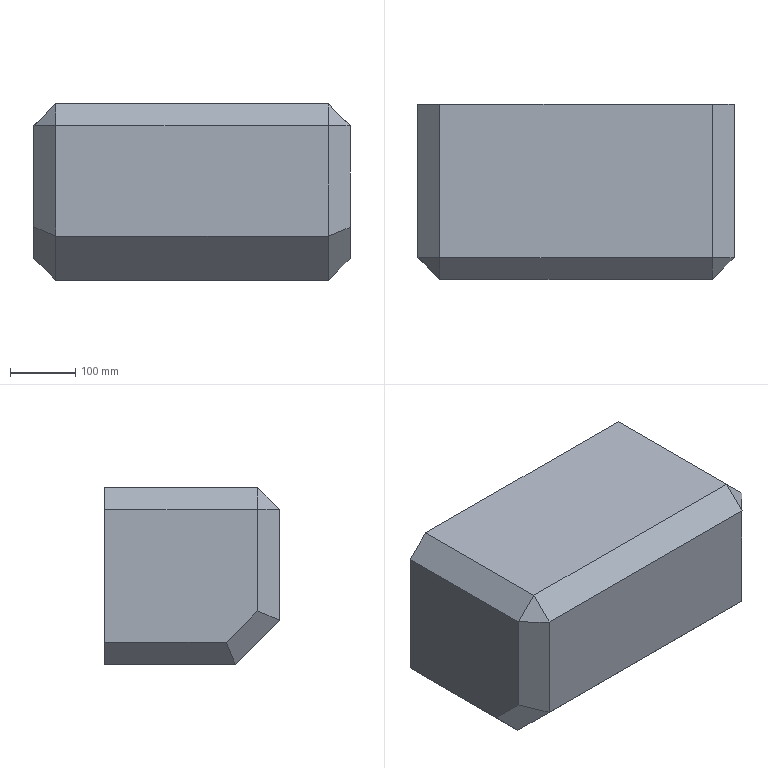Part | SolidWorks | features BaseBody 1 | 1 solid | 35 faces | box 484.18 x 267.622 x 270.437 mm | volume 1846046 mm3 | plane 35
STEP:
#1=CARTESIAN_POINT('',(-212.465,-140.024,-218.661));
#2=VERTEX_POINT('',#1);
#3=CARTESIAN_POINT('',(204.537,-140.008,-219.009));
#4=VERTEX_POINT('',#3);
#5=CARTESIAN_POINT('',(-212.465,-140.024,-218.661));
#6=DIRECTION('',(1.,0.00003864,-0.0008339));
#7=VECTOR('',#6,1000.);
#8=LINE('',#5,#7);
#9=EDGE_CURVE('',#2,#4,#8,.T.);
#10=ORIENTED_EDGE('',*,*,#9,.T.);
#11=CARTESIAN_POINT('',(204.679,-140.083,-49.863));
#12=VERTEX_POINT('',#11);
#13=CARTESIAN_POINT('',(204.679,-140.083,-49.863));
#14=DIRECTION('',(-0.0008339,0.0004454,-1.));
#15=VECTOR('',#14,1000.);
#16=LINE('',#13,#15);
#17=EDGE_CURVE('',#12,#4,#16,.T.);
#18=ORIENTED_EDGE('',*,*,#17,.F.);
#19=CARTESIAN_POINT('',(-212.323,-140.099,-49.515));
#20=VERTEX_POINT('',#19);
#21=CARTESIAN_POINT('',(-212.323,-140.099,-49.515));
#22=DIRECTION('',(1.,0.00003864,-0.0008339));
#23=VECTOR('',#22,1000.);
#24=LINE('',#21,#23);
#25=EDGE_CURVE('',#20,#12,#24,.T.);
#26=ORIENTED_EDGE('',*,*,#25,.F.);
#27=CARTESIAN_POINT('',(-212.323,-140.099,-49.515));
#28=DIRECTION('',(-0.0008339,0.0004454,-1.));
#29=VECTOR('',#28,1000.);
#30=LINE('',#27,#29);
#31=EDGE_CURVE('',#20,#2,#30,.T.);
#32=ORIENTED_EDGE('',*,*,#31,.T.);
#33=EDGE_LOOP('',(#10,#18,#26,#32));
#34=FACE_OUTER_BOUND('',#33,.T.);
#35=CARTESIAN_POINT('',(15.017,-140.064,-109.221));
#36=DIRECTION('',(-0.00003827,1.,0.0004455));
#37=DIRECTION('',(0.9963,0.,0.08559));
#38=AXIS2_PLACEMENT_3D('',#35,#36,#37);
#39=PLANE('',#38);
#40=ADVANCED_FACE('',(#34),#39,.F.);
#41=CARTESIAN_POINT('',(-245.65,-106.775,-49.472));
#42=VERTEX_POINT('',#41);
#43=CARTESIAN_POINT('',(-245.825,-106.6,-49.647));
#44=VERTEX_POINT('',#43);
#45=CARTESIAN_POINT('',(-245.65,-106.775,-49.472));
#46=DIRECTION('',(-0.5779,0.5776,-0.5766));
#47=VECTOR('',#46,1000.);
#48=LINE('',#45,#47);
#49=EDGE_CURVE('',#42,#44,#48,.T.);
#50=ORIENTED_EDGE('',*,*,#49,.T.);
#51=CARTESIAN_POINT('',(-245.954,-106.531,-204.742));
#52=VERTEX_POINT('',#51);
#53=CARTESIAN_POINT('',(-245.954,-106.531,-204.742));
#54=DIRECTION('',(0.0008339,-0.0004454,1.));
#55=VECTOR('',#54,1000.);
#56=LINE('',#53,#55);
#57=EDGE_CURVE('',#52,#44,#56,.T.);
#58=ORIENTED_EDGE('',*,*,#57,.F.);
#59=CARTESIAN_POINT('',(-245.954,-106.531,-204.742));
#60=DIRECTION('',(0.6784,-0.6784,-0.282));
#61=VECTOR('',#60,1000.);
#62=LINE('',#59,#61);
#63=EDGE_CURVE('',#52,#2,#62,.T.);
#64=ORIENTED_EDGE('',*,*,#63,.T.);
#65=ORIENTED_EDGE('',*,*,#31,.F.);
#66=CARTESIAN_POINT('',(-212.323,-140.099,-49.515));
#67=DIRECTION('',(-0.7071,0.7071,0.0009047));
#68=VECTOR('',#67,1000.);
#69=LINE('',#66,#68);
#70=EDGE_CURVE('',#20,#42,#69,.T.);
#71=ORIENTED_EDGE('',*,*,#70,.T.);
#72=EDGE_LOOP('',(#50,#58,#64,#65,#71));
#73=FACE_OUTER_BOUND('',#72,.T.);
#74=CARTESIAN_POINT('',(-212.465,-140.024,-218.661));
#75=DIRECTION('',(0.7071,0.7071,-0.0002747));
#76=DIRECTION('',(-0.0003885,0.,-1.));
#77=AXIS2_PLACEMENT_3D('',#74,#75,#76);
#78=PLANE('',#77);
#79=ADVANCED_FACE('',(#73),#78,.F.);
#80=CARTESIAN_POINT('',(-212.297,-106.789,-16.175));
#81=VERTEX_POINT('',#80);
#82=CARTESIAN_POINT('',(-212.323,-140.099,-49.515));
#83=DIRECTION('',(0.0005626,0.7068,0.7074));
#84=VECTOR('',#83,1000.);
#85=LINE('',#82,#84);
#86=EDGE_CURVE('',#20,#81,#85,.T.);
#87=ORIENTED_EDGE('',*,*,#86,.T.);
#88=CARTESIAN_POINT('',(-245.65,-106.775,-49.472));
#89=DIRECTION('',(0.7077,-0.0002876,0.7065));
#90=VECTOR('',#89,1000.);
#91=LINE('',#88,#90);
#92=EDGE_CURVE('',#42,#81,#91,.T.);
#93=ORIENTED_EDGE('',*,*,#92,.F.);
#94=ORIENTED_EDGE('',*,*,#70,.F.);
#95=EDGE_LOOP('',(#87,#93,#94));
#96=FACE_OUTER_BOUND('',#95,.T.);
#97=CARTESIAN_POINT('',(-212.323,-140.099,-49.515));
#98=DIRECTION('',(0.5768,0.5776,-0.5776));
#99=DIRECTION('',(-0.7076,0.,-0.7067));
#100=AXIS2_PLACEMENT_3D('',#97,#98,#99);
#101=PLANE('',#100);
#102=ADVANCED_FACE('',(#96),#101,.F.);
#103=CARTESIAN_POINT('',(-212.306,127.386,-16.071));
#104=VERTEX_POINT('',#103);
#105=CARTESIAN_POINT('',(-212.306,127.386,-16.071));
#106=DIRECTION('',(0.00003827,-1.,-0.0004455));
#107=VECTOR('',#106,1000.);
#108=LINE('',#105,#107);
#109=EDGE_CURVE('',#104,#81,#108,.T.);
#110=ORIENTED_EDGE('',*,*,#109,.F.);
#111=CARTESIAN_POINT('',(-245.834,127.4,-49.543));
#112=VERTEX_POINT('',#111);
#113=CARTESIAN_POINT('',(-212.306,127.386,-16.071));
#114=DIRECTION('',(-0.7077,0.0002876,-0.7065));
#115=VECTOR('',#114,1000.);
#116=LINE('',#113,#115);
#117=EDGE_CURVE('',#104,#112,#116,.T.);
#118=ORIENTED_EDGE('',*,*,#117,.T.);
#119=CARTESIAN_POINT('',(-245.834,127.4,-49.543));
#120=DIRECTION('',(0.00003827,-1.,-0.0004455));
#121=VECTOR('',#120,1000.);
#122=LINE('',#119,#121);
#123=EDGE_CURVE('',#112,#44,#122,.T.);
#124=ORIENTED_EDGE('',*,*,#123,.T.);
#125=ORIENTED_EDGE('',*,*,#49,.F.);
#126=ORIENTED_EDGE('',*,*,#92,.T.);
#127=EDGE_LOOP('',(#110,#118,#124,#125,#126));
#128=FACE_OUTER_BOUND('',#127,.T.);
#129=CARTESIAN_POINT('',(-257.333,-154.78,-61.159));
#130=DIRECTION('',(0.7065,0.0003423,-0.7077));
#131=DIRECTION('',(0.,-1.,-0.0004837));
#132=AXIS2_PLACEMENT_3D('',#129,#130,#131);
#133=PLANE('',#132);
#134=ADVANCED_FACE('',(#128),#133,.F.);
#135=ORIENTED_EDGE('',*,*,#57,.T.);
#136=ORIENTED_EDGE('',*,*,#123,.F.);
#137=CARTESIAN_POINT('',(-246.003,127.49,-252.543));
#138=VERTEX_POINT('',#137);
#139=CARTESIAN_POINT('',(-245.834,127.4,-49.543));
#140=DIRECTION('',(-0.0008339,0.0004454,-1.));
#141=VECTOR('',#140,1000.);
#142=LINE('',#139,#141);
#143=EDGE_CURVE('',#112,#138,#142,.T.);
#144=ORIENTED_EDGE('',*,*,#143,.T.);
#145=CARTESIAN_POINT('',(-245.996,-58.605,-252.626));
#146=VERTEX_POINT('',#145);
#147=CARTESIAN_POINT('',(-246.003,127.49,-252.543));
#148=DIRECTION('',(0.00003827,-1.,-0.0004455));
#149=VECTOR('',#148,1000.);
#150=LINE('',#147,#149);
#151=EDGE_CURVE('',#138,#146,#150,.T.);
#152=ORIENTED_EDGE('',*,*,#151,.T.);
#153=CARTESIAN_POINT('',(-245.954,-106.531,-204.742));
#154=DIRECTION('',(-0.0006167,0.7074,-0.7068));
#155=VECTOR('',#154,1000.);
#156=LINE('',#153,#155);
#157=EDGE_CURVE('',#52,#146,#156,.T.);
#158=ORIENTED_EDGE('',*,*,#157,.F.);
#159=EDGE_LOOP('',(#135,#136,#144,#152,#158));
#160=FACE_OUTER_BOUND('',#159,.T.);
#161=CARTESIAN_POINT('',(-245.995,-140.009,-255.236));
#162=DIRECTION('',(-1.,-0.00003864,0.0008339));
#163=DIRECTION('',(-0.00003864,1.,0.));
#164=AXIS2_PLACEMENT_3D('',#161,#162,#163);
#165=PLANE('',#164);
#166=ADVANCED_FACE('',(#160),#165,.T.);
#167=CARTESIAN_POINT('',(-212.523,-72.465,-286.16));
#168=VERTEX_POINT('',#167);
#169=CARTESIAN_POINT('',(-245.996,-58.605,-252.626));
#170=DIRECTION('',(0.678,-0.2808,-0.6793));
#171=VECTOR('',#170,1000.);
#172=LINE('',#169,#171);
#173=EDGE_CURVE('',#146,#168,#172,.T.);
#174=ORIENTED_EDGE('',*,*,#173,.T.);
#175=CARTESIAN_POINT('',(-212.523,-72.465,-286.16));
#176=DIRECTION('',(0.0006167,-0.7074,0.7068));
#177=VECTOR('',#176,1000.);
#178=LINE('',#175,#177);
#179=EDGE_CURVE('',#168,#2,#178,.T.);
#180=ORIENTED_EDGE('',*,*,#179,.T.);
#181=ORIENTED_EDGE('',*,*,#63,.F.);
#182=ORIENTED_EDGE('',*,*,#157,.T.);
#183=EDGE_LOOP('',(#174,#180,#181,#182));
#184=FACE_OUTER_BOUND('',#183,.T.);
#185=CARTESIAN_POINT('',(-212.523,-72.465,-286.16));
#186=DIRECTION('',(0.7075,0.4998,0.4996));
#187=DIRECTION('',(0.,0.707,-0.7072));
#188=AXIS2_PLACEMENT_3D('',#185,#186,#187);
#189=PLANE('',#188);
#190=ADVANCED_FACE('',(#184),#189,.F.);
#191=ORIENTED_EDGE('',*,*,#9,.F.);
#192=ORIENTED_EDGE('',*,*,#179,.F.);
#193=CARTESIAN_POINT('',(204.479,-72.449,-286.508));
#194=VERTEX_POINT('',#193);
#195=CARTESIAN_POINT('',(-212.523,-72.465,-286.16));
#196=DIRECTION('',(1.,0.00003864,-0.0008339));
#197=VECTOR('',#196,1000.);
#198=LINE('',#195,#197);
#199=EDGE_CURVE('',#168,#194,#198,.T.);
#200=ORIENTED_EDGE('',*,*,#199,.T.);
#201=CARTESIAN_POINT('',(204.479,-72.449,-286.508));
#202=DIRECTION('',(0.0006167,-0.7074,0.7068));
#203=VECTOR('',#202,1000.);
#204=LINE('',#201,#203);
#205=EDGE_CURVE('',#194,#4,#204,.T.);
#206=ORIENTED_EDGE('',*,*,#205,.T.);
#207=EDGE_LOOP('',(#191,#192,#200,#206));
#208=FACE_OUTER_BOUND('',#207,.T.);
#209=CARTESIAN_POINT('',(-299.167,-140.027,-218.589));
#210=DIRECTION('',(0.0005626,0.7068,0.7074));
#211=DIRECTION('',(1.,-0.000796,0.));
#212=AXIS2_PLACEMENT_3D('',#209,#210,#211);
#213=PLANE('',#212);
#214=ADVANCED_FACE('',(#208),#213,.F.);
#215=CARTESIAN_POINT('',(238.048,-106.513,-205.146));
#216=VERTEX_POINT('',#215);
#217=CARTESIAN_POINT('',(238.048,-106.513,-205.146));
#218=DIRECTION('',(-0.6788,-0.6785,-0.2808));
#219=VECTOR('',#218,1000.);
#220=LINE('',#217,#219);
#221=EDGE_CURVE('',#216,#4,#220,.T.);
#222=ORIENTED_EDGE('',*,*,#221,.T.);
#223=ORIENTED_EDGE('',*,*,#205,.F.);
#224=CARTESIAN_POINT('',(238.006,-58.586,-253.029));
#225=VERTEX_POINT('',#224);
#226=CARTESIAN_POINT('',(238.006,-58.586,-253.029));
#227=DIRECTION('',(-0.6792,-0.2808,-0.6782));
#228=VECTOR('',#227,1000.);
#229=LINE('',#226,#228);
#230=EDGE_CURVE('',#225,#194,#229,.T.);
#231=ORIENTED_EDGE('',*,*,#230,.F.);
#232=CARTESIAN_POINT('',(238.006,-58.586,-253.029));
#233=DIRECTION('',(0.0006167,-0.7074,0.7068));
#234=VECTOR('',#233,1000.);
#235=LINE('',#232,#234);
#236=EDGE_CURVE('',#225,#216,#235,.T.);
#237=ORIENTED_EDGE('',*,*,#236,.T.);
#238=EDGE_LOOP('',(#222,#223,#231,#237));
#239=FACE_OUTER_BOUND('',#238,.T.);
#240=CARTESIAN_POINT('',(204.479,-72.449,-286.508));
#241=DIRECTION('',(0.7067,-0.4997,-0.5008));
#242=DIRECTION('',(0.,-0.7079,0.7064));
#243=AXIS2_PLACEMENT_3D('',#240,#241,#242);
#244=PLANE('',#243);
#245=ADVANCED_FACE('',(#239),#244,.T.);
#246=CARTESIAN_POINT('',(237.999,127.509,-252.946));
#247=VERTEX_POINT('',#246);
#248=CARTESIAN_POINT('',(237.999,127.509,-252.946));
#249=DIRECTION('',(0.00003827,-1.,-0.0004455));
#250=VECTOR('',#249,1000.);
#251=LINE('',#248,#250);
#252=EDGE_CURVE('',#247,#225,#251,.T.);
#253=ORIENTED_EDGE('',*,*,#252,.F.);
#254=CARTESIAN_POINT('',(238.168,127.418,-49.946));
#255=VERTEX_POINT('',#254);
#256=CARTESIAN_POINT('',(237.999,127.509,-252.946));
#257=DIRECTION('',(0.0008339,-0.0004454,1.));
#258=VECTOR('',#257,1000.);
#259=LINE('',#256,#258);
#260=EDGE_CURVE('',#247,#255,#259,.T.);
#261=ORIENTED_EDGE('',*,*,#260,.T.);
#262=CARTESIAN_POINT('',(238.177,-106.582,-50.051));
#263=VERTEX_POINT('',#262);
#264=CARTESIAN_POINT('',(238.168,127.418,-49.946));
#265=DIRECTION('',(0.00003827,-1.,-0.0004455));
#266=VECTOR('',#265,1000.);
#267=LINE('',#264,#266);
#268=EDGE_CURVE('',#255,#263,#267,.T.);
#269=ORIENTED_EDGE('',*,*,#268,.T.);
#270=CARTESIAN_POINT('',(238.048,-106.513,-205.146));
#271=DIRECTION('',(0.0008339,-0.0004454,1.));
#272=VECTOR('',#271,1000.);
#273=LINE('',#270,#272);
#274=EDGE_CURVE('',#216,#263,#273,.T.);
#275=ORIENTED_EDGE('',*,*,#274,.F.);
#276=ORIENTED_EDGE('',*,*,#236,.F.);
#277=EDGE_LOOP('',(#253,#261,#269,#275,#276));
#278=FACE_OUTER_BOUND('',#277,.T.);
#279=CARTESIAN_POINT('',(238.184,-140.085,-43.658));
#280=DIRECTION('',(1.,0.00003864,-0.0008339));
#281=DIRECTION('',(0.,-0.9989,-0.04628));
#282=AXIS2_PLACEMENT_3D('',#279,#280,#281);
#283=PLANE('',#282);
#284=ADVANCED_FACE('',(#278),#283,.T.);
#285=ORIENTED_EDGE('',*,*,#17,.T.);
#286=ORIENTED_EDGE('',*,*,#221,.F.);
#287=ORIENTED_EDGE('',*,*,#274,.T.);
#288=CARTESIAN_POINT('',(238.002,-106.757,-49.876));
#289=VERTEX_POINT('',#288);
#290=CARTESIAN_POINT('',(238.002,-106.757,-49.876));
#291=DIRECTION('',(0.5768,0.5776,-0.5776));
#292=VECTOR('',#291,1000.);
#293=LINE('',#290,#292);
#294=EDGE_CURVE('',#289,#263,#293,.T.);
#295=ORIENTED_EDGE('',*,*,#294,.F.);
#296=CARTESIAN_POINT('',(238.002,-106.757,-49.876));
#297=DIRECTION('',(-0.7071,-0.7071,0.0002747));
#298=VECTOR('',#297,1000.);
#299=LINE('',#296,#298);
#300=EDGE_CURVE('',#289,#12,#299,.T.);
#301=ORIENTED_EDGE('',*,*,#300,.T.);
#302=EDGE_LOOP('',(#285,#286,#287,#295,#301));
#303=FACE_OUTER_BOUND('',#302,.T.);
#304=CARTESIAN_POINT('',(204.537,-140.008,-219.009));
#305=DIRECTION('',(0.7071,-0.7071,-0.0009047));
#306=DIRECTION('',(0.,0.001279,-1.));
#307=AXIS2_PLACEMENT_3D('',#304,#305,#306);
#308=PLANE('',#307);
#309=ADVANCED_FACE('',(#303),#308,.T.);
#310=CARTESIAN_POINT('',(204.705,-106.773,-16.523));
#311=VERTEX_POINT('',#310);
#312=CARTESIAN_POINT('',(204.679,-140.083,-49.863));
#313=DIRECTION('',(0.0005626,0.7068,0.7074));
#314=VECTOR('',#313,1000.);
#315=LINE('',#312,#314);
#316=EDGE_CURVE('',#12,#311,#315,.T.);
#317=ORIENTED_EDGE('',*,*,#316,.F.);
#318=ORIENTED_EDGE('',*,*,#300,.F.);
#319=CARTESIAN_POINT('',(204.705,-106.773,-16.523));
#320=DIRECTION('',(0.7065,0.0003423,-0.7077));
#321=VECTOR('',#320,1000.);
#322=LINE('',#319,#321);
#323=EDGE_CURVE('',#311,#289,#322,.T.);
#324=ORIENTED_EDGE('',*,*,#323,.F.);
#325=EDGE_LOOP('',(#317,#318,#324));
#326=FACE_OUTER_BOUND('',#325,.T.);
#327=CARTESIAN_POINT('',(204.679,-140.083,-49.863));
#328=DIRECTION('',(0.5779,-0.5776,0.5766));
#329=DIRECTION('',(0.,-0.7065,-0.7077));
#330=AXIS2_PLACEMENT_3D('',#327,#328,#329);
#331=PLANE('',#330);
#332=ADVANCED_FACE('',(#326),#331,.T.);
#333=ORIENTED_EDGE('',*,*,#294,.T.);
#334=ORIENTED_EDGE('',*,*,#268,.F.);
#335=CARTESIAN_POINT('',(204.696,127.402,-16.419));
#336=VERTEX_POINT('',#335);
#337=CARTESIAN_POINT('',(238.168,127.418,-49.946));
#338=DIRECTION('',(-0.7065,-0.0003423,0.7077));
#339=VECTOR('',#338,1000.);
#340=LINE('',#337,#339);
#341=EDGE_CURVE('',#255,#336,#340,.T.);
#342=ORIENTED_EDGE('',*,*,#341,.T.);
#343=CARTESIAN_POINT('',(204.696,127.402,-16.419));
#344=DIRECTION('',(0.00003827,-1.,-0.0004455));
#345=VECTOR('',#344,1000.);
#346=LINE('',#343,#345);
#347=EDGE_CURVE('',#336,#311,#346,.T.);
#348=ORIENTED_EDGE('',*,*,#347,.T.);
#349=ORIENTED_EDGE('',*,*,#323,.T.);
#350=EDGE_LOOP('',(#333,#334,#342,#348,#349));
#351=FACE_OUTER_BOUND('',#350,.T.);
#352=CARTESIAN_POINT('',(249.669,-154.761,-61.582));
#353=DIRECTION('',(0.7077,-0.0002876,0.7065));
#354=DIRECTION('',(0.,-1.,-0.0004071));
#355=AXIS2_PLACEMENT_3D('',#352,#353,#354);
#356=PLANE('',#355);
#357=ADVANCED_FACE('',(#351),#356,.T.);
#358=CARTESIAN_POINT('',(204.705,-106.773,-16.523));
#359=DIRECTION('',(-1.,-0.00003864,0.0008339));
#360=VECTOR('',#359,1000.);
#361=LINE('',#358,#360);
#362=EDGE_CURVE('',#311,#81,#361,.T.);
#363=ORIENTED_EDGE('',*,*,#362,.F.);
#364=ORIENTED_EDGE('',*,*,#347,.F.);
#365=CARTESIAN_POINT('',(204.696,127.402,-16.419));
#366=DIRECTION('',(-1.,-0.00003864,0.0008339));
#367=VECTOR('',#366,1000.);
#368=LINE('',#365,#367);
#369=EDGE_CURVE('',#336,#104,#368,.T.);
#370=ORIENTED_EDGE('',*,*,#369,.T.);
#371=ORIENTED_EDGE('',*,*,#109,.T.);
#372=EDGE_LOOP('',(#363,#364,#370,#371));
#373=FACE_OUTER_BOUND('',#372,.T.);
#374=CARTESIAN_POINT('',(-214.698,-140.114,-16.188));
#375=DIRECTION('',(0.0008339,-0.0004454,1.));
#376=DIRECTION('',(-0.4711,-0.8821,0.));
#377=AXIS2_PLACEMENT_3D('',#374,#375,#376);
#378=PLANE('',#377);
#379=ADVANCED_FACE('',(#373),#378,.T.);
#380=CARTESIAN_POINT('',(-241.835,127.4,-51.203));
#381=VERTEX_POINT('',#380);
#382=CARTESIAN_POINT('',(-210.652,127.388,-20.072));
#383=VERTEX_POINT('',#382);
#384=CARTESIAN_POINT('',(-241.835,127.4,-51.203));
#385=DIRECTION('',(0.7077,-0.0002876,0.7065));
#386=VECTOR('',#385,1000.);
#387=LINE('',#384,#386);
#388=EDGE_CURVE('',#381,#383,#387,.T.);
#389=ORIENTED_EDGE('',*,*,#388,.F.);
#390=CARTESIAN_POINT('',(-242.002,127.489,-250.889));
#391=VERTEX_POINT('',#390);
#392=CARTESIAN_POINT('',(-241.835,127.4,-51.203));
#393=DIRECTION('',(-0.0008339,0.0004454,-1.));
#394=VECTOR('',#393,1000.);
#395=LINE('',#392,#394);
#396=EDGE_CURVE('',#381,#391,#395,.T.);
#397=ORIENTED_EDGE('',*,*,#396,.T.);
#398=CARTESIAN_POINT('',(-210.871,127.505,-282.072));
#399=VERTEX_POINT('',#398);
#400=CARTESIAN_POINT('',(-210.871,127.505,-282.072));
#401=DIRECTION('',(-0.7065,-0.0003423,0.7077));
#402=VECTOR('',#401,1000.);
#403=LINE('',#400,#402);
#404=EDGE_CURVE('',#399,#391,#403,.T.);
#405=ORIENTED_EDGE('',*,*,#404,.F.);
#406=CARTESIAN_POINT('',(202.817,127.52,-282.417));
#407=VERTEX_POINT('',#406);
#408=CARTESIAN_POINT('',(-210.871,127.505,-282.072));
#409=DIRECTION('',(1.,0.00003864,-0.0008339));
#410=VECTOR('',#409,1000.);
#411=LINE('',#408,#410);
#412=EDGE_CURVE('',#399,#407,#411,.T.);
#413=ORIENTED_EDGE('',*,*,#412,.T.);
#414=CARTESIAN_POINT('',(234.,127.508,-251.286));
#415=VERTEX_POINT('',#414);
#416=CARTESIAN_POINT('',(234.,127.508,-251.286));
#417=DIRECTION('',(-0.7077,0.0002876,-0.7065));
#418=VECTOR('',#417,1000.);
#419=LINE('',#416,#418);
#420=EDGE_CURVE('',#415,#407,#419,.T.);
#421=ORIENTED_EDGE('',*,*,#420,.F.);
#422=CARTESIAN_POINT('',(234.167,127.419,-51.6));
#423=VERTEX_POINT('',#422);
#424=CARTESIAN_POINT('',(234.,127.508,-251.286));
#425=DIRECTION('',(0.0008339,-0.0004454,1.));
#426=VECTOR('',#425,1000.);
#427=LINE('',#424,#426);
#428=EDGE_CURVE('',#415,#423,#427,.T.);
#429=ORIENTED_EDGE('',*,*,#428,.T.);
#430=CARTESIAN_POINT('',(203.036,127.404,-20.417));
#431=VERTEX_POINT('',#430);
#432=CARTESIAN_POINT('',(203.036,127.404,-20.417));
#433=DIRECTION('',(0.7065,0.0003423,-0.7077));
#434=VECTOR('',#433,1000.);
#435=LINE('',#432,#434);
#436=EDGE_CURVE('',#431,#423,#435,.T.);
#437=ORIENTED_EDGE('',*,*,#436,.F.);
#438=CARTESIAN_POINT('',(203.036,127.404,-20.417));
#439=DIRECTION('',(-1.,-0.00003864,0.0008339));
#440=VECTOR('',#439,1000.);
#441=LINE('',#438,#440);
#442=EDGE_CURVE('',#431,#383,#441,.T.);
#443=ORIENTED_EDGE('',*,*,#442,.T.);
#444=EDGE_LOOP('',(#389,#397,#405,#413,#421,#429,#437,#443));
#445=FACE_BOUND('',#444,.T.);
#446=CARTESIAN_POINT('',(-212.531,127.506,-286.071));
#447=VERTEX_POINT('',#446);
#448=CARTESIAN_POINT('',(204.471,127.522,-286.418));
#449=VERTEX_POINT('',#448);
#450=CARTESIAN_POINT('',(-212.531,127.506,-286.071));
#451=DIRECTION('',(1.,0.00003864,-0.0008339));
#452=VECTOR('',#451,1000.);
#453=LINE('',#450,#452);
#454=EDGE_CURVE('',#447,#449,#453,.T.);
#455=ORIENTED_EDGE('',*,*,#454,.F.);
#456=CARTESIAN_POINT('',(-246.003,127.49,-252.543));
#457=DIRECTION('',(0.7065,0.0003423,-0.7077));
#458=VECTOR('',#457,1000.);
#459=LINE('',#456,#458);
#460=EDGE_CURVE('',#138,#447,#459,.T.);
#461=ORIENTED_EDGE('',*,*,#460,.F.);
#462=ORIENTED_EDGE('',*,*,#143,.F.);
#463=ORIENTED_EDGE('',*,*,#117,.F.);
#464=ORIENTED_EDGE('',*,*,#369,.F.);
#465=ORIENTED_EDGE('',*,*,#341,.F.);
#466=ORIENTED_EDGE('',*,*,#260,.F.);
#467=CARTESIAN_POINT('',(204.471,127.522,-286.418));
#468=DIRECTION('',(0.7077,-0.0002876,0.7065));
#469=VECTOR('',#468,1000.);
#470=LINE('',#467,#469);
#471=EDGE_CURVE('',#449,#247,#470,.T.);
#472=ORIENTED_EDGE('',*,*,#471,.F.);
#473=EDGE_LOOP('',(#455,#461,#462,#463,#464,#465,#466,#472));
#474=FACE_OUTER_BOUND('',#473,.T.);
#475=CARTESIAN_POINT('',(15.007,127.436,-109.102));
#476=DIRECTION('',(-0.00003827,1.,0.0004455));
#477=DIRECTION('',(0.9963,0.,0.08559));
#478=AXIS2_PLACEMENT_3D('',#475,#476,#477);
#479=PLANE('',#478);
#480=ADVANCED_FACE('',(#445,#474),#479,.T.);
#481=CARTESIAN_POINT('',(204.471,127.522,-286.418));
#482=DIRECTION('',(0.00003827,-1.,-0.0004455));
#483=VECTOR('',#482,1000.);
#484=LINE('',#481,#483);
#485=EDGE_CURVE('',#449,#194,#484,.T.);
#486=ORIENTED_EDGE('',*,*,#485,.F.);
#487=ORIENTED_EDGE('',*,*,#471,.T.);
#488=ORIENTED_EDGE('',*,*,#252,.T.);
#489=ORIENTED_EDGE('',*,*,#230,.T.);
#490=EDGE_LOOP('',(#486,#487,#488,#489));
#491=FACE_OUTER_BOUND('',#490,.T.);
#492=CARTESIAN_POINT('',(204.482,-154.662,-286.544));
#493=DIRECTION('',(0.7065,0.0003423,-0.7077));
#494=DIRECTION('',(0.,-1.,-0.0004837));
#495=AXIS2_PLACEMENT_3D('',#492,#493,#494);
#496=PLANE('',#495);
#497=ADVANCED_FACE('',(#491),#496,.T.);
#498=ORIENTED_EDGE('',*,*,#199,.F.);
#499=CARTESIAN_POINT('',(-212.531,127.506,-286.071));
#500=DIRECTION('',(0.00003827,-1.,-0.0004455));
#501=VECTOR('',#500,1000.);
#502=LINE('',#499,#501);
#503=EDGE_CURVE('',#447,#168,#502,.T.);
#504=ORIENTED_EDGE('',*,*,#503,.F.);
#505=ORIENTED_EDGE('',*,*,#454,.T.);
#506=ORIENTED_EDGE('',*,*,#485,.T.);
#507=EDGE_LOOP('',(#498,#504,#505,#506));
#508=FACE_OUTER_BOUND('',#507,.T.);
#509=CARTESIAN_POINT('',(207.057,-139.978,-286.54));
#510=DIRECTION('',(-0.0008339,0.0004454,-1.));
#511=DIRECTION('',(-1.,0.,0.0008339));
#512=AXIS2_PLACEMENT_3D('',#509,#510,#511);
#513=PLANE('',#512);
#514=ADVANCED_FACE('',(#508),#513,.T.);
#515=ORIENTED_EDGE('',*,*,#151,.F.);
#516=ORIENTED_EDGE('',*,*,#460,.T.);
#517=ORIENTED_EDGE('',*,*,#503,.T.);
#518=ORIENTED_EDGE('',*,*,#173,.F.);
#519=EDGE_LOOP('',(#515,#516,#517,#518));
#520=FACE_OUTER_BOUND('',#519,.T.);
#521=CARTESIAN_POINT('',(-212.52,-154.678,-286.196));
#522=DIRECTION('',(0.7077,-0.0002876,0.7065));
#523=DIRECTION('',(0.,-1.,-0.0004071));
#524=AXIS2_PLACEMENT_3D('',#521,#522,#523);
#525=PLANE('',#524);
#526=ADVANCED_FACE('',(#520),#525,.F.);
#527=CARTESIAN_POINT('',(203.045,-105.114,-20.521));
#528=VERTEX_POINT('',#527);
#529=CARTESIAN_POINT('',(203.036,127.404,-20.417));
#530=DIRECTION('',(0.00003827,-1.,-0.0004455));
#531=VECTOR('',#530,1000.);
#532=LINE('',#529,#531);
#533=EDGE_CURVE('',#431,#528,#532,.T.);
#534=ORIENTED_EDGE('',*,*,#533,.T.);
#535=CARTESIAN_POINT('',(-210.644,-105.13,-20.176));
#536=VERTEX_POINT('',#535);
#537=CARTESIAN_POINT('',(203.045,-105.114,-20.521));
#538=DIRECTION('',(-1.,-0.00003864,0.0008339));
#539=VECTOR('',#538,1000.);
#540=LINE('',#537,#539);
#541=EDGE_CURVE('',#528,#536,#540,.T.);
#542=ORIENTED_EDGE('',*,*,#541,.T.);
#543=CARTESIAN_POINT('',(-210.652,127.388,-20.072));
#544=DIRECTION('',(0.00003827,-1.,-0.0004455));
#545=VECTOR('',#544,1000.);
#546=LINE('',#543,#545);
#547=EDGE_CURVE('',#383,#536,#546,.T.);
#548=ORIENTED_EDGE('',*,*,#547,.F.);
#549=ORIENTED_EDGE('',*,*,#442,.F.);
#550=EDGE_LOOP('',(#534,#542,#548,#549));
#551=FACE_OUTER_BOUND('',#550,.T.);
#552=CARTESIAN_POINT('',(-214.701,-140.112,-20.188));
#553=DIRECTION('',(0.0008339,-0.0004454,1.));
#554=DIRECTION('',(-0.4711,-0.8821,0.));
#555=AXIS2_PLACEMENT_3D('',#552,#553,#554);
#556=PLANE('',#555);
#557=ADVANCED_FACE('',(#551),#556,.F.);
#558=ORIENTED_EDGE('',*,*,#547,.T.);
#559=CARTESIAN_POINT('',(-211.029,-105.516,-20.561));
#560=VERTEX_POINT('',#559);
#561=CARTESIAN_POINT('',(-210.644,-105.13,-20.176));
#562=DIRECTION('',(-0.5778,-0.5771,-0.5771));
#563=VECTOR('',#562,1000.);
#564=LINE('',#561,#563);
#565=EDGE_CURVE('',#536,#560,#564,.T.);
#566=ORIENTED_EDGE('',*,*,#565,.T.);
#567=CARTESIAN_POINT('',(-241.265,-105.503,-50.747));
#568=VERTEX_POINT('',#567);
#569=CARTESIAN_POINT('',(-211.029,-105.516,-20.561));
#570=DIRECTION('',(-0.7077,0.0002876,-0.7065));
#571=VECTOR('',#570,1000.);
#572=LINE('',#569,#571);
#573=EDGE_CURVE('',#560,#568,#572,.T.);
#574=ORIENTED_EDGE('',*,*,#573,.T.);
#575=CARTESIAN_POINT('',(-241.826,-104.943,-51.307));
#576=VERTEX_POINT('',#575);
#577=CARTESIAN_POINT('',(-241.265,-105.503,-50.747));
#578=DIRECTION('',(-0.5779,0.5776,-0.5766));
#579=VECTOR('',#578,1000.);
#580=LINE('',#577,#579);
#581=EDGE_CURVE('',#568,#576,#580,.T.);
#582=ORIENTED_EDGE('',*,*,#581,.T.);
#583=CARTESIAN_POINT('',(-241.835,127.4,-51.203));
#584=DIRECTION('',(0.00003827,-1.,-0.0004455));
#585=VECTOR('',#584,1000.);
#586=LINE('',#583,#585);
#587=EDGE_CURVE('',#381,#576,#586,.T.);
#588=ORIENTED_EDGE('',*,*,#587,.F.);
#589=ORIENTED_EDGE('',*,*,#388,.T.);
#590=EDGE_LOOP('',(#558,#566,#574,#582,#588,#589));
#591=FACE_OUTER_BOUND('',#590,.T.);
#592=CARTESIAN_POINT('',(-254.507,-154.779,-63.99));
#593=DIRECTION('',(0.7065,0.0003423,-0.7077));
#594=DIRECTION('',(0.,-1.,-0.0004837));
#595=AXIS2_PLACEMENT_3D('',#592,#593,#594);
#596=PLANE('',#595);
#597=ADVANCED_FACE('',(#591),#596,.T.);
#598=ORIENTED_EDGE('',*,*,#587,.T.);
#599=CARTESIAN_POINT('',(-241.954,-104.875,-204.058));
#600=VERTEX_POINT('',#599);
#601=CARTESIAN_POINT('',(-241.954,-104.875,-204.058));
#602=DIRECTION('',(0.0008339,-0.0004454,1.));
#603=VECTOR('',#602,1000.);
#604=LINE('',#601,#603);
#605=EDGE_CURVE('',#600,#576,#604,.T.);
#606=ORIENTED_EDGE('',*,*,#605,.F.);
#607=CARTESIAN_POINT('',(-241.995,-57.919,-250.972));
#608=VERTEX_POINT('',#607);
#609=CARTESIAN_POINT('',(-241.995,-57.919,-250.972));
#610=DIRECTION('',(0.0006167,-0.7074,0.7068));
#611=VECTOR('',#610,1000.);
#612=LINE('',#609,#611);
#613=EDGE_CURVE('',#608,#600,#612,.T.);
#614=ORIENTED_EDGE('',*,*,#613,.F.);
#615=CARTESIAN_POINT('',(-242.002,127.489,-250.889));
#616=DIRECTION('',(0.00003827,-1.,-0.0004455));
#617=VECTOR('',#616,1000.);
#618=LINE('',#615,#617);
#619=EDGE_CURVE('',#391,#608,#618,.T.);
#620=ORIENTED_EDGE('',*,*,#619,.F.);
#621=ORIENTED_EDGE('',*,*,#396,.F.);
#622=EDGE_LOOP('',(#598,#606,#614,#620,#621));
#623=FACE_OUTER_BOUND('',#622,.T.);
#624=CARTESIAN_POINT('',(-241.995,-140.009,-255.239));
#625=DIRECTION('',(-1.,-0.00003864,0.0008339));
#626=DIRECTION('',(-0.00003864,1.,0.));
#627=AXIS2_PLACEMENT_3D('',#624,#625,#626);
#628=PLANE('',#627);
#629=ADVANCED_FACE('',(#623),#628,.F.);
#630=ORIENTED_EDGE('',*,*,#619,.T.);
#631=CARTESIAN_POINT('',(-210.863,-70.81,-282.16));
#632=VERTEX_POINT('',#631);
#633=CARTESIAN_POINT('',(-241.995,-57.919,-250.972));
#634=DIRECTION('',(0.678,-0.2808,-0.6793));
#635=VECTOR('',#634,1000.);
#636=LINE('',#633,#635);
#637=EDGE_CURVE('',#608,#632,#636,.T.);
#638=ORIENTED_EDGE('',*,*,#637,.T.);
#639=CARTESIAN_POINT('',(-210.871,127.505,-282.072));
#640=DIRECTION('',(0.00003827,-1.,-0.0004455));
#641=VECTOR('',#640,1000.);
#642=LINE('',#639,#641);
#643=EDGE_CURVE('',#399,#632,#642,.T.);
#644=ORIENTED_EDGE('',*,*,#643,.F.);
#645=ORIENTED_EDGE('',*,*,#404,.T.);
#646=EDGE_LOOP('',(#630,#638,#644,#645));
#647=FACE_OUTER_BOUND('',#646,.T.);
#648=CARTESIAN_POINT('',(-209.69,-154.679,-283.37));
#649=DIRECTION('',(0.7077,-0.0002876,0.7065));
#650=DIRECTION('',(0.,-1.,-0.0004071));
#651=AXIS2_PLACEMENT_3D('',#648,#649,#650);
#652=PLANE('',#651);
#653=ADVANCED_FACE('',(#647),#652,.T.);
#654=ORIENTED_EDGE('',*,*,#643,.T.);
#655=CARTESIAN_POINT('',(202.825,-70.794,-282.505));
#656=VERTEX_POINT('',#655);
#657=CARTESIAN_POINT('',(-210.863,-70.81,-282.16));
#658=DIRECTION('',(1.,0.00003864,-0.0008339));
#659=VECTOR('',#658,1000.);
#660=LINE('',#657,#659);
#661=EDGE_CURVE('',#632,#656,#660,.T.);
#662=ORIENTED_EDGE('',*,*,#661,.T.);
#663=CARTESIAN_POINT('',(202.817,127.52,-282.417));
#664=DIRECTION('',(0.00003827,-1.,-0.0004455));
#665=VECTOR('',#664,1000.);
#666=LINE('',#663,#665);
#667=EDGE_CURVE('',#407,#656,#666,.T.);
#668=ORIENTED_EDGE('',*,*,#667,.F.);
#669=ORIENTED_EDGE('',*,*,#412,.F.);
#670=EDGE_LOOP('',(#654,#662,#668,#669));
#671=FACE_OUTER_BOUND('',#670,.T.);
#672=CARTESIAN_POINT('',(207.06,-139.979,-282.54));
#673=DIRECTION('',(-0.0008339,0.0004454,-1.));
#674=DIRECTION('',(-1.,0.,0.0008339));
#675=AXIS2_PLACEMENT_3D('',#672,#673,#674);
#676=PLANE('',#675);
#677=ADVANCED_FACE('',(#671),#676,.F.);
#678=ORIENTED_EDGE('',*,*,#667,.T.);
#679=CARTESIAN_POINT('',(234.007,-57.901,-251.369));
#680=VERTEX_POINT('',#679);
#681=CARTESIAN_POINT('',(234.007,-57.901,-251.369));
#682=DIRECTION('',(-0.6792,-0.2808,-0.6782));
#683=VECTOR('',#682,1000.);
#684=LINE('',#681,#683);
#685=EDGE_CURVE('',#680,#656,#684,.T.);
#686=ORIENTED_EDGE('',*,*,#685,.F.);
#687=CARTESIAN_POINT('',(234.,127.508,-251.286));
#688=DIRECTION('',(0.00003827,-1.,-0.0004455));
#689=VECTOR('',#688,1000.);
#690=LINE('',#687,#689);
#691=EDGE_CURVE('',#415,#680,#690,.T.);
#692=ORIENTED_EDGE('',*,*,#691,.F.);
#693=ORIENTED_EDGE('',*,*,#420,.T.);
#694=EDGE_LOOP('',(#678,#686,#692,#693));
#695=FACE_OUTER_BOUND('',#694,.T.);
#696=CARTESIAN_POINT('',(201.656,-154.663,-283.713));
#697=DIRECTION('',(0.7065,0.0003423,-0.7077));
#698=DIRECTION('',(0.,-1.,-0.0004837));
#699=AXIS2_PLACEMENT_3D('',#696,#697,#698);
#700=PLANE('',#699);
#701=ADVANCED_FACE('',(#695),#700,.F.);
#702=ORIENTED_EDGE('',*,*,#691,.T.);
#703=CARTESIAN_POINT('',(234.048,-104.856,-204.455));
#704=VERTEX_POINT('',#703);
#705=CARTESIAN_POINT('',(234.048,-104.856,-204.455));
#706=DIRECTION('',(-0.0006167,0.7074,-0.7068));
#707=VECTOR('',#706,1000.);
#708=LINE('',#705,#707);
#709=EDGE_CURVE('',#704,#680,#708,.T.);
#710=ORIENTED_EDGE('',*,*,#709,.F.);
#711=CARTESIAN_POINT('',(234.176,-104.924,-51.704));
#712=VERTEX_POINT('',#711);
#713=CARTESIAN_POINT('',(234.048,-104.856,-204.455));
#714=DIRECTION('',(0.0008339,-0.0004454,1.));
#715=VECTOR('',#714,1000.);
#716=LINE('',#713,#715);
#717=EDGE_CURVE('',#704,#712,#716,.T.);
#718=ORIENTED_EDGE('',*,*,#717,.T.);
#719=CARTESIAN_POINT('',(234.167,127.419,-51.6));
#720=DIRECTION('',(0.00003827,-1.,-0.0004455));
#721=VECTOR('',#720,1000.);
#722=LINE('',#719,#721);
#723=EDGE_CURVE('',#423,#712,#722,.T.);
#724=ORIENTED_EDGE('',*,*,#723,.F.);
#725=ORIENTED_EDGE('',*,*,#428,.F.);
#726=EDGE_LOOP('',(#702,#710,#718,#724,#725));
#727=FACE_OUTER_BOUND('',#726,.T.);
#728=CARTESIAN_POINT('',(234.184,-140.085,-43.654));
#729=DIRECTION('',(1.,0.00003864,-0.0008339));
#730=DIRECTION('',(0.,-0.9989,-0.04628));
#731=AXIS2_PLACEMENT_3D('',#728,#729,#730);
#732=PLANE('',#731);
#733=ADVANCED_FACE('',(#727),#732,.F.);
#734=ORIENTED_EDGE('',*,*,#723,.T.);
#735=CARTESIAN_POINT('',(233.616,-105.485,-51.143));
#736=VERTEX_POINT('',#735);
#737=CARTESIAN_POINT('',(233.616,-105.485,-51.143));
#738=DIRECTION('',(0.5768,0.5776,-0.5776));
#739=VECTOR('',#738,1000.);
#740=LINE('',#737,#739);
#741=EDGE_CURVE('',#736,#712,#740,.T.);
#742=ORIENTED_EDGE('',*,*,#741,.F.);
#743=CARTESIAN_POINT('',(203.43,-105.5,-20.907));
#744=VERTEX_POINT('',#743);
#745=CARTESIAN_POINT('',(233.616,-105.485,-51.143));
#746=DIRECTION('',(-0.7065,-0.0003423,0.7077));
#747=VECTOR('',#746,1000.);
#748=LINE('',#745,#747);
#749=EDGE_CURVE('',#736,#744,#748,.T.);
#750=ORIENTED_EDGE('',*,*,#749,.T.);
#751=CARTESIAN_POINT('',(203.045,-105.114,-20.521));
#752=DIRECTION('',(0.5769,-0.5771,-0.5781));
#753=VECTOR('',#752,1000.);
#754=LINE('',#751,#753);
#755=EDGE_CURVE('',#528,#744,#754,.T.);
#756=ORIENTED_EDGE('',*,*,#755,.F.);
#757=ORIENTED_EDGE('',*,*,#533,.F.);
#758=ORIENTED_EDGE('',*,*,#436,.T.);
#759=EDGE_LOOP('',(#734,#742,#750,#756,#757,#758));
#760=FACE_OUTER_BOUND('',#759,.T.);
#761=CARTESIAN_POINT('',(246.839,-154.759,-64.408));
#762=DIRECTION('',(0.7077,-0.0002876,0.7065));
#763=DIRECTION('',(0.,-1.,-0.0004071));
#764=AXIS2_PLACEMENT_3D('',#761,#762,#763);
#765=PLANE('',#764);
#766=ADVANCED_FACE('',(#760),#765,.F.);
#767=ORIENTED_EDGE('',*,*,#565,.F.);
#768=ORIENTED_EDGE('',*,*,#541,.F.);
#769=ORIENTED_EDGE('',*,*,#755,.T.);
#770=CARTESIAN_POINT('',(203.406,-135.697,-51.131));
#771=VERTEX_POINT('',#770);
#772=CARTESIAN_POINT('',(203.406,-135.697,-51.131));
#773=DIRECTION('',(0.0005626,0.7068,0.7074));
#774=VECTOR('',#773,1000.);
#775=LINE('',#772,#774);
#776=EDGE_CURVE('',#771,#744,#775,.T.);
#777=ORIENTED_EDGE('',*,*,#776,.F.);
#778=CARTESIAN_POINT('',(203.02,-136.082,-51.516));
#779=VERTEX_POINT('',#778);
#780=CARTESIAN_POINT('',(203.02,-136.082,-51.516));
#781=DIRECTION('',(0.5778,0.5771,0.5771));
#782=VECTOR('',#781,1000.);
#783=LINE('',#780,#782);
#784=EDGE_CURVE('',#779,#771,#783,.T.);
#785=ORIENTED_EDGE('',*,*,#784,.F.);
#786=CARTESIAN_POINT('',(-210.668,-136.098,-51.171));
#787=VERTEX_POINT('',#786);
#788=CARTESIAN_POINT('',(-210.668,-136.098,-51.171));
#789=DIRECTION('',(1.,0.00003864,-0.0008339));
#790=VECTOR('',#789,1000.);
#791=LINE('',#788,#790);
#792=EDGE_CURVE('',#787,#779,#791,.T.);
#793=ORIENTED_EDGE('',*,*,#792,.F.);
#794=CARTESIAN_POINT('',(-211.053,-135.713,-50.785));
#795=VERTEX_POINT('',#794);
#796=CARTESIAN_POINT('',(-210.668,-136.098,-51.171));
#797=DIRECTION('',(-0.5769,0.5771,0.5781));
#798=VECTOR('',#797,1000.);
#799=LINE('',#796,#798);
#800=EDGE_CURVE('',#787,#795,#799,.T.);
#801=ORIENTED_EDGE('',*,*,#800,.T.);
#802=CARTESIAN_POINT('',(-211.053,-135.713,-50.785));
#803=DIRECTION('',(0.0005626,0.7068,0.7074));
#804=VECTOR('',#803,1000.);
#805=LINE('',#802,#804);
#806=EDGE_CURVE('',#795,#560,#805,.T.);
#807=ORIENTED_EDGE('',*,*,#806,.T.);
#808=EDGE_LOOP('',(#767,#768,#769,#777,#785,#793,#801,#807));
#809=FACE_OUTER_BOUND('',#808,.T.);
#810=CARTESIAN_POINT('',(-299.002,-103.963,-18.93));
#811=DIRECTION('',(-0.0006167,0.7074,-0.7068));
#812=DIRECTION('',(-1.,0.,0.0008726));
#813=AXIS2_PLACEMENT_3D('',#810,#811,#812);
#814=PLANE('',#813);
#815=ADVANCED_FACE('',(#809),#814,.T.);
#816=ORIENTED_EDGE('',*,*,#573,.F.);
#817=ORIENTED_EDGE('',*,*,#806,.F.);
#818=CARTESIAN_POINT('',(-241.265,-105.503,-50.747));
#819=DIRECTION('',(0.7071,-0.7071,-0.0009047));
#820=VECTOR('',#819,1000.);
#821=LINE('',#818,#820);
#822=EDGE_CURVE('',#568,#795,#821,.T.);
#823=ORIENTED_EDGE('',*,*,#822,.F.);
#824=EDGE_LOOP('',(#816,#817,#823));
#825=FACE_OUTER_BOUND('',#824,.T.);
#826=CARTESIAN_POINT('',(-210.016,-137.789,-51.825));
#827=DIRECTION('',(0.5768,0.5776,-0.5776));
#828=DIRECTION('',(-0.7076,0.,-0.7067));
#829=AXIS2_PLACEMENT_3D('',#826,#827,#828);
#830=PLANE('',#829);
#831=ADVANCED_FACE('',(#825),#830,.T.);
#832=ORIENTED_EDGE('',*,*,#800,.F.);
#833=CARTESIAN_POINT('',(-210.806,-136.025,-217.004));
#834=VERTEX_POINT('',#833);
#835=CARTESIAN_POINT('',(-210.668,-136.098,-51.171));
#836=DIRECTION('',(-0.0008339,0.0004454,-1.));
#837=VECTOR('',#836,1000.);
#838=LINE('',#835,#837);
#839=EDGE_CURVE('',#787,#834,#838,.T.);
#840=ORIENTED_EDGE('',*,*,#839,.T.);
#841=CARTESIAN_POINT('',(-241.954,-104.875,-204.058));
#842=DIRECTION('',(0.6784,-0.6784,-0.282));
#843=VECTOR('',#842,1000.);
#844=LINE('',#841,#843);
#845=EDGE_CURVE('',#600,#834,#844,.T.);
#846=ORIENTED_EDGE('',*,*,#845,.F.);
#847=ORIENTED_EDGE('',*,*,#605,.T.);
#848=ORIENTED_EDGE('',*,*,#581,.F.);
#849=ORIENTED_EDGE('',*,*,#822,.T.);
#850=EDGE_LOOP('',(#832,#840,#846,#847,#848,#849));
#851=FACE_OUTER_BOUND('',#850,.T.);
#852=CARTESIAN_POINT('',(-209.636,-137.195,-218.662));
#853=DIRECTION('',(0.7071,0.7071,-0.0002747));
#854=DIRECTION('',(-0.0003885,0.,-1.));
#855=AXIS2_PLACEMENT_3D('',#852,#853,#854);
#856=PLANE('',#855);
#857=ADVANCED_FACE('',(#851),#856,.T.);
#858=ORIENTED_EDGE('',*,*,#845,.T.);
#859=CARTESIAN_POINT('',(-210.863,-70.81,-282.16));
#860=DIRECTION('',(0.0006167,-0.7074,0.7068));
#861=VECTOR('',#860,1000.);
#862=LINE('',#859,#861);
#863=EDGE_CURVE('',#632,#834,#862,.T.);
#864=ORIENTED_EDGE('',*,*,#863,.F.);
#865=ORIENTED_EDGE('',*,*,#637,.F.);
#866=ORIENTED_EDGE('',*,*,#613,.T.);
#867=EDGE_LOOP('',(#858,#864,#865,#866));
#868=FACE_OUTER_BOUND('',#867,.T.);
#869=CARTESIAN_POINT('',(-209.693,-70.466,-284.161));
#870=DIRECTION('',(0.7075,0.4998,0.4996));
#871=DIRECTION('',(0.,0.707,-0.7072));
#872=AXIS2_PLACEMENT_3D('',#869,#870,#871);
#873=PLANE('',#872);
#874=ADVANCED_FACE('',(#868),#873,.T.);
#875=ORIENTED_EDGE('',*,*,#661,.F.);
#876=ORIENTED_EDGE('',*,*,#863,.T.);
#877=CARTESIAN_POINT('',(202.882,-136.009,-217.349));
#878=VERTEX_POINT('',#877);
#879=CARTESIAN_POINT('',(-210.806,-136.025,-217.004));
#880=DIRECTION('',(1.,0.00003864,-0.0008339));
#881=VECTOR('',#880,1000.);
#882=LINE('',#879,#881);
#883=EDGE_CURVE('',#834,#878,#882,.T.);
#884=ORIENTED_EDGE('',*,*,#883,.T.);
#885=CARTESIAN_POINT('',(202.825,-70.794,-282.505));
#886=DIRECTION('',(0.0006167,-0.7074,0.7068));
#887=VECTOR('',#886,1000.);
#888=LINE('',#885,#887);
#889=EDGE_CURVE('',#656,#878,#888,.T.);
#890=ORIENTED_EDGE('',*,*,#889,.F.);
#891=EDGE_LOOP('',(#875,#876,#884,#890));
#892=FACE_OUTER_BOUND('',#891,.T.);
#893=CARTESIAN_POINT('',(-299.165,-137.2,-215.759));
#894=DIRECTION('',(0.0005626,0.7068,0.7074));
#895=DIRECTION('',(1.,-0.000796,0.));
#896=AXIS2_PLACEMENT_3D('',#893,#894,#895);
#897=PLANE('',#896);
#898=ADVANCED_FACE('',(#892),#897,.T.);
#899=ORIENTED_EDGE('',*,*,#685,.T.);
#900=ORIENTED_EDGE('',*,*,#889,.T.);
#901=CARTESIAN_POINT('',(234.048,-104.856,-204.455));
#902=DIRECTION('',(-0.6788,-0.6785,-0.2808));
#903=VECTOR('',#902,1000.);
#904=LINE('',#901,#903);
#905=EDGE_CURVE('',#704,#878,#904,.T.);
#906=ORIENTED_EDGE('',*,*,#905,.F.);
#907=ORIENTED_EDGE('',*,*,#709,.T.);
#908=EDGE_LOOP('',(#899,#900,#906,#907));
#909=FACE_OUTER_BOUND('',#908,.T.);
#910=CARTESIAN_POINT('',(201.652,-70.45,-284.504));
#911=DIRECTION('',(0.7067,-0.4997,-0.5008));
#912=DIRECTION('',(0.,-0.7079,0.7064));
#913=AXIS2_PLACEMENT_3D('',#910,#911,#912);
#914=PLANE('',#913);
#915=ADVANCED_FACE('',(#909),#914,.F.);
#916=ORIENTED_EDGE('',*,*,#741,.T.);
#917=ORIENTED_EDGE('',*,*,#717,.F.);
#918=ORIENTED_EDGE('',*,*,#905,.T.);
#919=CARTESIAN_POINT('',(203.02,-136.082,-51.516));
#920=DIRECTION('',(-0.0008339,0.0004454,-1.));
#921=VECTOR('',#920,1000.);
#922=LINE('',#919,#921);
#923=EDGE_CURVE('',#779,#878,#922,.T.);
#924=ORIENTED_EDGE('',*,*,#923,.F.);
#925=ORIENTED_EDGE('',*,*,#784,.T.);
#926=CARTESIAN_POINT('',(203.406,-135.697,-51.131));
#927=DIRECTION('',(0.7071,0.7071,-0.0002747));
#928=VECTOR('',#927,1000.);
#929=LINE('',#926,#928);
#930=EDGE_CURVE('',#771,#736,#929,.T.);
#931=ORIENTED_EDGE('',*,*,#930,.T.);
#932=EDGE_LOOP('',(#916,#917,#918,#924,#925,#931));
#933=FACE_OUTER_BOUND('',#932,.T.);
#934=CARTESIAN_POINT('',(201.709,-137.179,-219.005));
#935=DIRECTION('',(0.7071,-0.7071,-0.0009047));
#936=DIRECTION('',(0.,0.001279,-1.));
#937=AXIS2_PLACEMENT_3D('',#934,#935,#936);
#938=PLANE('',#937);
#939=ADVANCED_FACE('',(#933),#938,.F.);
#940=ORIENTED_EDGE('',*,*,#930,.F.);
#941=ORIENTED_EDGE('',*,*,#776,.T.);
#942=ORIENTED_EDGE('',*,*,#749,.F.);
#943=EDGE_LOOP('',(#940,#941,#942));
#944=FACE_OUTER_BOUND('',#943,.T.);
#945=CARTESIAN_POINT('',(202.367,-137.773,-52.169));
#946=DIRECTION('',(0.5779,-0.5776,0.5766));
#947=DIRECTION('',(0.,-0.7065,-0.7077));
#948=AXIS2_PLACEMENT_3D('',#945,#946,#947);
#949=PLANE('',#948);
#950=ADVANCED_FACE('',(#944),#949,.F.);
#951=ORIENTED_EDGE('',*,*,#792,.T.);
#952=ORIENTED_EDGE('',*,*,#923,.T.);
#953=ORIENTED_EDGE('',*,*,#883,.F.);
#954=ORIENTED_EDGE('',*,*,#839,.F.);
#955=EDGE_LOOP('',(#951,#952,#953,#954));
#956=FACE_OUTER_BOUND('',#955,.T.);
#957=CARTESIAN_POINT('',(15.017,-136.064,-109.219));
#958=DIRECTION('',(-0.00003827,1.,0.0004455));
#959=DIRECTION('',(0.9963,0.,0.08559));
#960=AXIS2_PLACEMENT_3D('',#957,#958,#959);
#961=PLANE('',#960);
#962=ADVANCED_FACE('',(#956),#961,.T.);
#963=ORIENTED_EDGE('',*,*,#25,.T.);
#964=ORIENTED_EDGE('',*,*,#316,.T.);
#965=ORIENTED_EDGE('',*,*,#362,.T.);
#966=ORIENTED_EDGE('',*,*,#86,.F.);
#967=EDGE_LOOP('',(#963,#964,#965,#966));
#968=FACE_OUTER_BOUND('',#967,.T.);
#969=CARTESIAN_POINT('',(-299.,-106.792,-16.103));
#970=DIRECTION('',(-0.0006167,0.7074,-0.7068));
#971=DIRECTION('',(-1.,0.,0.0008726));
#972=AXIS2_PLACEMENT_3D('',#969,#970,#971);
#973=PLANE('',#972);
#974=ADVANCED_FACE('',(#968),#973,.F.);
#975=CLOSED_SHELL('',(#40,#79,#102,#134,#166,#190,#214,#245,#284,#309,#332,#357,#379,#480,#497,#514,#526,#557,#597,#629,#653,#677,#701,#733,#766,#815,#831,#857,#874,#898,#915,#939,#950,#962,#974));
#976=MANIFOLD_SOLID_BREP('',#975);
#977=CARTESIAN_POINT('',(0.,0.,0.));
#978=DIRECTION('',(0.,0.,1.));
#979=DIRECTION('',(1.,0.,0.));
#980=AXIS2_PLACEMENT_3D('',#977,#978,#979);
#981=(LENGTH_UNIT()NAMED_UNIT(*)SI_UNIT(.MILLI.,.METRE.));
#982=UNCERTAINTY_MEASURE_WITH_UNIT(LENGTH_MEASURE(0.00001),#981,'','');
#983=(NAMED_UNIT(*)PLANE_ANGLE_UNIT()SI_UNIT($,.RADIAN.));
#984=(NAMED_UNIT(*)SI_UNIT($,.STERADIAN.)SOLID_ANGLE_UNIT());
#985=(GEOMETRIC_REPRESENTATION_CONTEXT(3)GLOBAL_UNCERTAINTY_ASSIGNED_CONTEXT((#982))GLOBAL_UNIT_ASSIGNED_CONTEXT((#981,#983,#984))REPRESENTATION_CONTEXT('',''));
#986=ADVANCED_BREP_SHAPE_REPRESENTATION('',(#976,#980),#985);